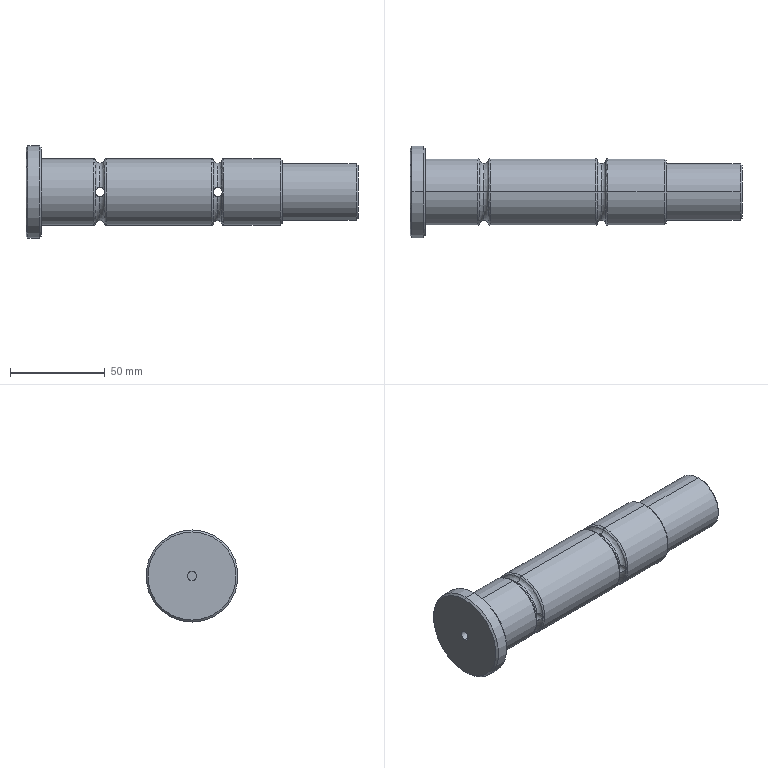Part | STEP file | PN_0001-01-07 Pin shaft B | 1 solid | 61 faces | box 175 x 48.5 x 48.5 mm | volume 160152 mm3 | cylinder 26 | torus 20 | cone 10 | plane 5 | commonest cylinder face diameters 4.8 x14 35 x6 5 x2 30 x2 48.5 x2